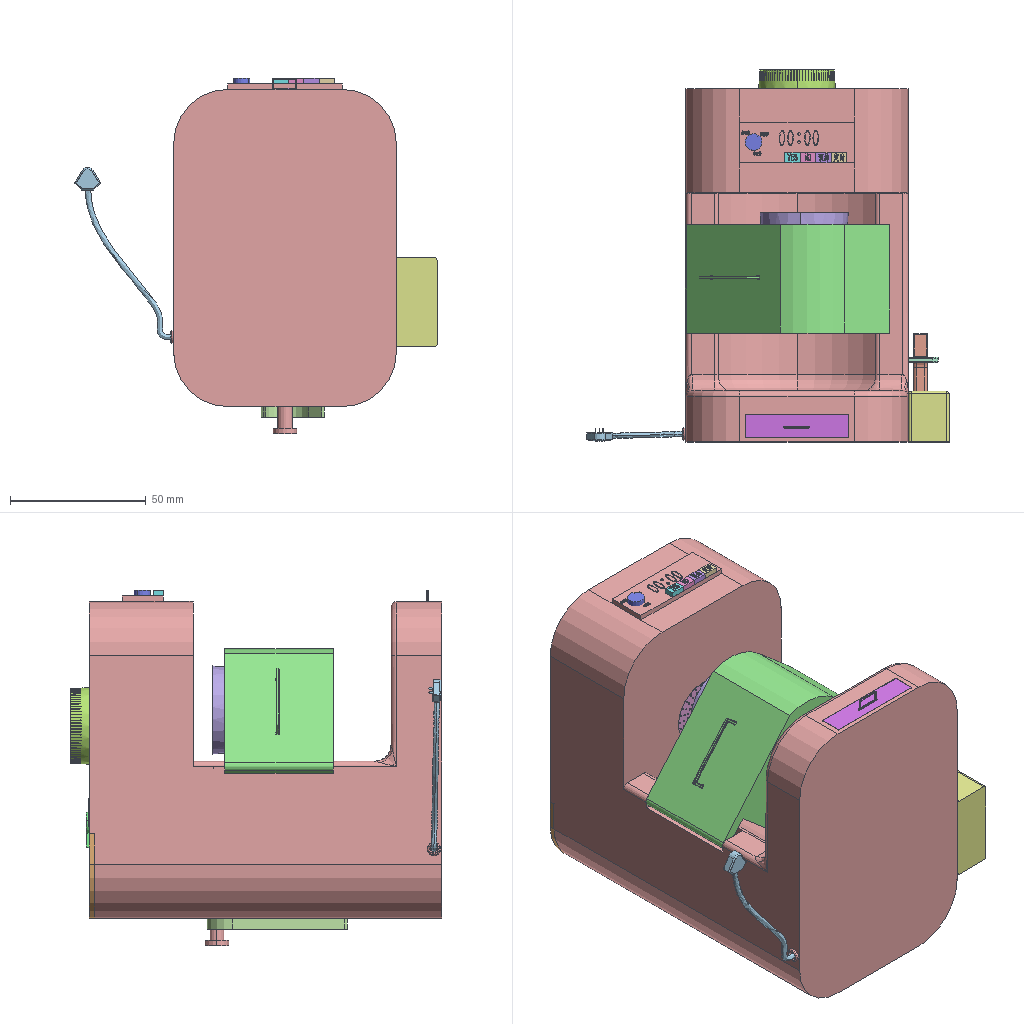Assembly | SolidWorks | 19 different items | 19 placed | box 133 x 137 x 131 mm
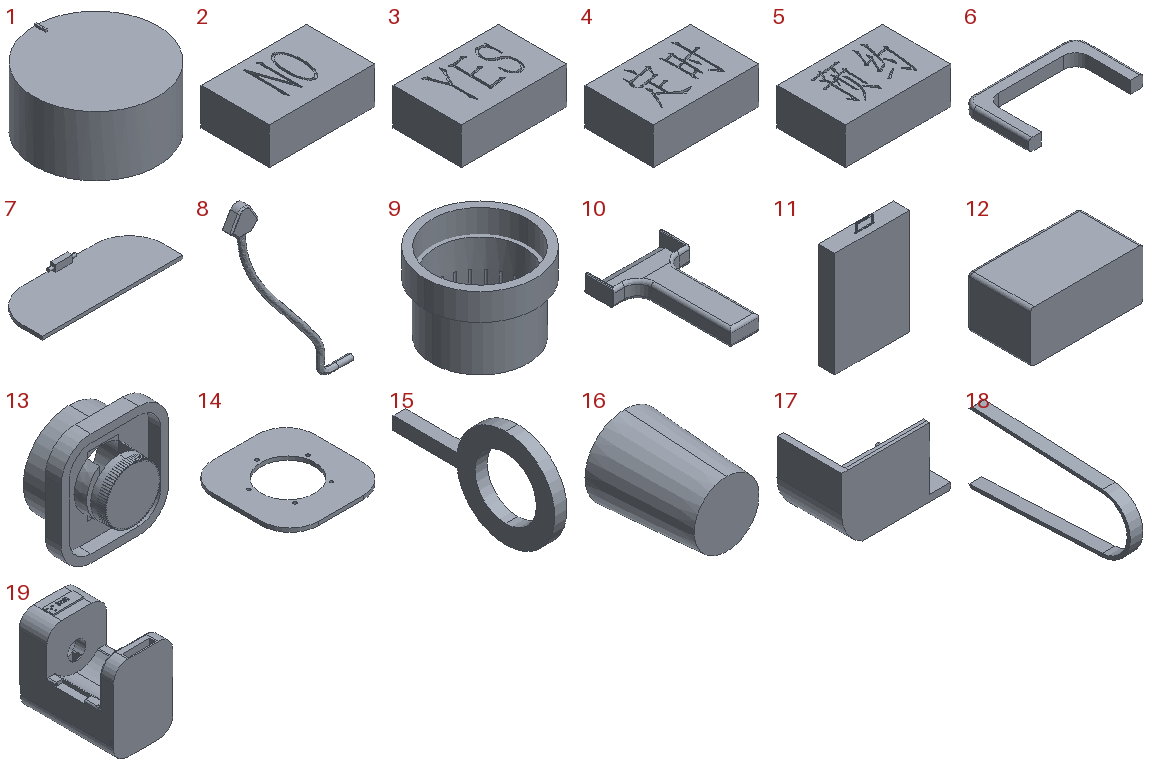Parts list (item | quantity | size | volume | features):
1 | x1 | 6.16 x 6.16 x 3.1 mm | 87.843 mm3 | features ICE 2, Extrusion 1
2 | x1 | 5.7 x 3.7 x 2 mm | 42.058 mm3 | features Extrusion 1, ICE 1
3 | x1 | 5.7 x 3.7 x 2 mm | 42.034 mm3 | features Extrusion 1, ICE 1
4 | x1 | 5.7 x 3.7 x 2 mm | 42.017 mm3 | features Extrusion 1, ICE 1
5 | x1 | 5.7 x 3.7 x 2 mm | 42.006 mm3 | features Extrusion 1, ICE 1
6 | x1 | 18.597 x 10.954 x 2 mm | 141.898 mm3 | features Fillet 2, ExtruThin 1
7 | x1 | 82.07 x 31.262 x 6 mm | 4923 mm3 | features ICE 2, Extrusion 1, MirrorPattern 1
8 | x1 | 41.382 x 4.5 x 63.54 mm | 377.613 mm3 | features Fillet 4, ICE 2, Chamfer 1, Sweep 1
9 | x1 | 29 x 29 x 20.3 mm | 2708 mm3 | features ICE 2, CirPattern 1, Extrusion 1, Shell 1
10 | x1 | 23 x 36.517 x 5 mm | 1470 mm3 | features Fillet 3, Chamfer 1, Extrusion 1, ICE 1
11 | x1 | 38.19 x 8.3 x 58 mm | 6865 mm3 | features Fillet 4, ICE 3, Extrusion 1
12 | x1 | 33 x 18.729 x 15 mm | 3493 mm3 | features Fillet 2, Extrusion 1, ICE 1
13 | x1 | 53.95 x 32 x 56.16 mm | 29305 mm3 | features ICE 6, CirPattern 1, CutThin 1, Extrusion 1
14 | x1 | 53.95 x 56.16 x 2 mm | 4376 mm3 | features ICE 2, CirPattern 1, Extrusion 1
15 | x1 | 1 x 13.171 x 8 mm | 36.178 mm3 | features Extrusion 1, ICE 1
16 | x1 | 32.541 x 42.384 x 32.541 mm | 8227 mm3 | features Revolution 1, Shell 1
17 | x1 | 67.531 x 44 x 48.042 mm | 19835 mm3 | features Fillet 5, BossThin 2, ICE 2, ExtruThin 1
18 | x1 | 4 x 51.055 x 22.562 mm | 440.681 mm3 | features Chamfer 2, ExtruThin 1
19 | x1 | 83.17 x 131 x 129.899 mm | 652006 mm3 | features ICE 30, Fillet 4, CirPattern 3, BossThin 2, Extrusion 1
Mates (type | each side: item.copy, entity, surface, feature):
Concentric | 19.1 face cylinder Cut-Extrude13 | 13.1 face cylinder Boss-Extrude2
Coincident | 19.1 face plane Cut-Extrude11 | 13.1 face plane Boss-Extrude1
Concentric | 19.1 face cylinder Cut-Extrude9 | 9.1 face cylinder Boss-Extrude1
Coincident | 19.1 face plane Cut-Extrude13 | 9.1 face plane Boss-Extrude2
Coincident | 19.1 face plane Cut-Extrude13 | 13.1 face plane Boss-Extrude2
Concentric | 13.1 face cone Boss-Extrude3 | 14.1 face cylinder Cut-Extrude1
Concentric | 19.1 face cylinder Cut-Extrude11 | 14.1 face cylinder Boss-Extrude1
Concentric | 19.1 face cylinder Cut-Extrude20 | 7.1 face cylinder Boss-Extrude6
Coincident | 19.1 face plane Cut-Extrude20 | 7.1 face plane Boss-Extrude6
Concentric | 19.1 face cylinder Cut-Extrude23 | 17.1 face cylinder Boss-Extrude1
Coincident | 19.1 face plane Cut-Extrude23 | 17.1 face plane Boss-Extrude1
Coincident | 16.1 face plane Revolve1 | 17.1 face plane Boss-Extrude2
Concentric | 16.1 edge | 17.1 edge
Coincident | 13.1 face plane Cut-Extrude4 | 14.1 face plane Boss-Extrude1
Coincident | 19.1 face plane Cut-Extrude15 | 7.1 face plane Boss-Extrude1
Concentric | 19.1 face cylinder Cut-Extrude24 | 8.1 face cylinder Sweep1
Coincident | 19.1 face plane Cut-Extrude24 | 8.1 face plane Sweep1
Coincident | 19.1 face plane Boss-Extrude1 | 12.1 face plane Boss-Extrude1 | 2 times
DistanceDim | 12.1 face plane Boss-Extrude1 | 19.1 face plane Cut-Extrude1
Coincident | 19.1 face plane Cut-Extrude25 | 11.1 face plane Boss-Extrude1
Coincident | 19.1 edge | 11.1 face plane Boss-Extrude1
Coincident | 19.1 face plane Cut-Extrude25 | 11.1 edge
DistanceDim | 12.1 face plane Boss-Extrude1 | 6.1 face plane Extrude-Thin1
DistanceDim | 6.1 face plane Extrude-Thin1 | 12.1 face plane Boss-Extrude1
Coincident | 6.1 face plane Extrude-Thin1 | 10.1 face plane Boss-Extrude1
Concentric | 19.1 face cylinder Boss-Extrude13 | 1.1 face cylinder Cut-Extrude1
Coincident | 19.1 face plane Boss-Extrude13 | 1.1 face plane Cut-Extrude1
Coincident | 19.1 face plane Boss-Extrude1 | 18.1 face plane Extrude-Thin1
Coincident | 12.1 face plane Cut-Extrude1 | 10.1 face plane Boss-Extrude1
DistanceDim | 10.1 face plane Boss-Extrude1 | 6.1 face plane Extrude-Thin1
Coincident | 19.1 face plane Boss-Extrude1 | 6.1 face plane Extrude-Thin1
Coincident | 19.1 face plane Boss-Extrude3 | 2.1 face plane Boss-Extrude1 | 2 times
Coincident | 19.1 face plane Boss-Extrude3 | 5.1 face plane Boss-Extrude1 | 2 times
Coincident | 19.1 face plane Boss-Extrude3 | 3.1 face plane Boss-Extrude1 | 2 times
Coincident | 19.1 face plane Boss-Extrude3 | 4.1 face plane Boss-Extrude1 | 2 times
Coincident | 2.1 edge | 3.1 edge
Coincident | 2.1 face plane Boss-Extrude1 | 5.1 edge
Coincident | 4.1 edge | 5.1 edge
Concentric | 19.1 face cylinder Boss-Extrude16 | 15.1 face cylinder Cut-Extrude1
Coincident | 19.1 face plane Boss-Extrude1 | 15.1 face plane Boss-Extrude2